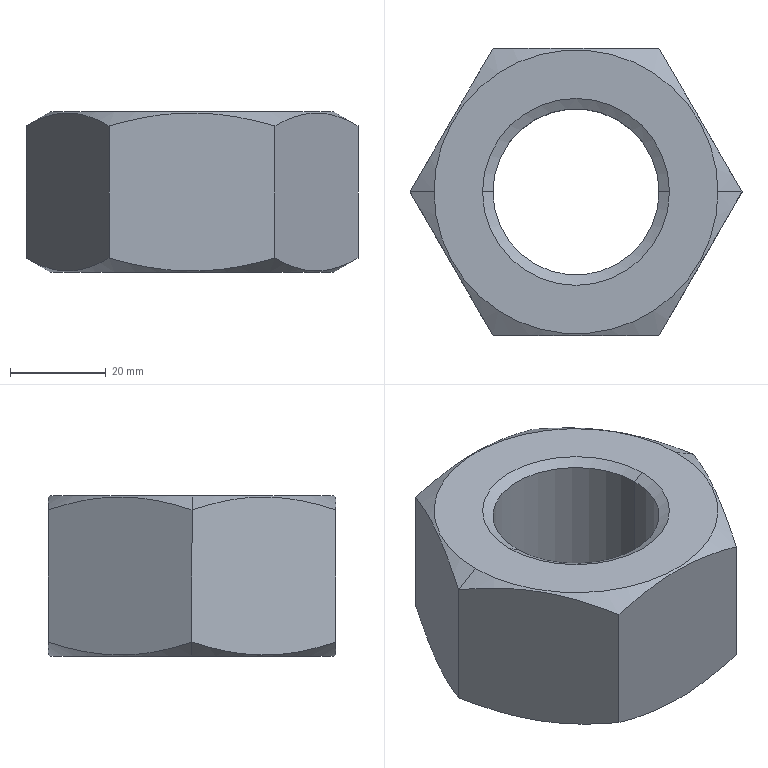Part | STEP file | hex nuts, style 1-grades ab gb(GB_FASTENER_NUT_SNAB1  B M39-N) | 1 solid | 18 faces | box 69.282 x 60 x 33.4 mm | volume 71685 mm3 | cone 8 | plane 8 | cylinder 2 | commonest cylinder face diameters 34.67 x2